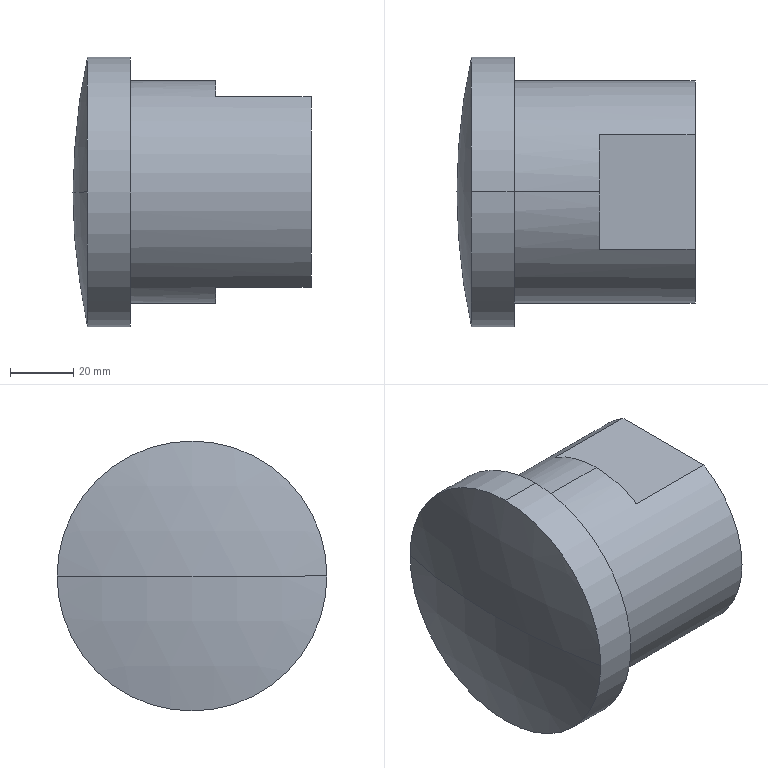Part | STEP file | OP10-028_cylinder connector (L) | 1 solid | 16 faces | box 75 x 85 x 85 mm | volume 251301 mm3 | cylinder 6 | plane 6 | cone 2 | sphere 2 | commonest cylinder face diameters 34.5 x2 70 x2 85 x2
STEP:
#1=CARTESIAN_POINT('',(0.,0.,0.));
#2=DIRECTION('',(0.,0.,1.));
#3=DIRECTION('',(1.,0.,0.));
#4=AXIS2_PLACEMENT_3D('',#1,#2,#3);
#5=CARTESIAN_POINT('',(-50.,0.,-17.25));
#6=VERTEX_POINT('',#5);
#7=CARTESIAN_POINT('',(0.,0.,-17.25));
#8=VERTEX_POINT('',#7);
#9=CARTESIAN_POINT('',(0.,0.,-17.25));
#10=DIRECTION('',(1.,0.,0.));
#11=VECTOR('',#10,1.);
#12=LINE('',#9,#11);
#13=CARTESIAN_POINT('',(0.,0.,0.));
#14=DIRECTION('',(1.,0.,0.));
#15=DIRECTION('',(0.,0.,-1.));
#16=AXIS2_PLACEMENT_3D('',#13,#14,#15);
#17=CYLINDRICAL_SURFACE('',#16,17.25);
#18=CARTESIAN_POINT('',(6.283,0.));
#19=DIRECTION('',(0.,1.));
#20=VECTOR('',#19,1.);
#21=LINE('',#18,#20);
#22=(GEOMETRIC_REPRESENTATION_CONTEXT(2)PARAMETRIC_REPRESENTATION_CONTEXT()REPRESENTATION_CONTEXT('',''));
#23=DEFINITIONAL_REPRESENTATION('',(#21),#22);
#24=PCURVE('',#17,#23);
#25=CARTESIAN_POINT('',(0.,0.,0.));
#26=DIRECTION('',(1.,0.,0.));
#27=DIRECTION('',(0.,0.,-1.));
#28=AXIS2_PLACEMENT_3D('',#25,#26,#27);
#29=CYLINDRICAL_SURFACE('',#28,17.25);
#30=CARTESIAN_POINT('',(0.,0.));
#31=DIRECTION('',(0.,1.));
#32=VECTOR('',#31,1.);
#33=LINE('',#30,#32);
#34=(GEOMETRIC_REPRESENTATION_CONTEXT(2)PARAMETRIC_REPRESENTATION_CONTEXT()REPRESENTATION_CONTEXT('',''));
#35=DEFINITIONAL_REPRESENTATION('',(#33),#34);
#36=PCURVE('',#29,#35);
#37=SURFACE_CURVE('',#12,(#24,#36),.PCURVE_S1.);
#38=EDGE_CURVE('',#6,#8,#37,.T.);
#39=ORIENTED_EDGE('',*,*,#38,.T.);
#40=CARTESIAN_POINT('',(0.,0.,17.25));
#41=VERTEX_POINT('',#40);
#42=CARTESIAN_POINT('',(0.,0.,0.));
#43=DIRECTION('',(1.,0.,0.));
#44=DIRECTION('',(0.,0.,-1.));
#45=AXIS2_PLACEMENT_3D('',#42,#43,#44);
#46=CIRCLE('',#45,17.25);
#47=CARTESIAN_POINT('',(0.,0.));
#48=DIRECTION('',(1.,0.));
#49=VECTOR('',#48,1.);
#50=LINE('',#47,#49);
#51=(GEOMETRIC_REPRESENTATION_CONTEXT(2)PARAMETRIC_REPRESENTATION_CONTEXT()REPRESENTATION_CONTEXT('',''));
#52=DEFINITIONAL_REPRESENTATION('',(#50),#51);
#53=PCURVE('',#17,#52);
#54=CARTESIAN_POINT('',(0.,0.,0.));
#55=DIRECTION('',(1.,0.,0.));
#56=DIRECTION('',(0.,0.,-1.));
#57=AXIS2_PLACEMENT_3D('',#54,#55,#56);
#58=PLANE('',#57);
#59=CARTESIAN_POINT('',(0.,0.));
#60=DIRECTION('',(1.,0.));
#61=AXIS2_PLACEMENT_2D('',#59,#60);
#62=CIRCLE('',#61,17.25);
#63=(GEOMETRIC_REPRESENTATION_CONTEXT(2)PARAMETRIC_REPRESENTATION_CONTEXT()REPRESENTATION_CONTEXT('',''));
#64=DEFINITIONAL_REPRESENTATION('',(#62),#63);
#65=PCURVE('',#58,#64);
#66=SURFACE_CURVE('',#46,(#53,#65),.PCURVE_S1.);
#67=EDGE_CURVE('',#41,#8,#66,.T.);
#68=ORIENTED_EDGE('',*,*,#67,.F.);
#69=CARTESIAN_POINT('',(-50.,0.,17.25));
#70=VERTEX_POINT('',#69);
#71=CARTESIAN_POINT('',(0.,0.,17.25));
#72=DIRECTION('',(1.,0.,0.));
#73=VECTOR('',#72,1.);
#74=LINE('',#71,#73);
#75=CARTESIAN_POINT('',(3.142,0.));
#76=DIRECTION('',(0.,1.));
#77=VECTOR('',#76,1.);
#78=LINE('',#75,#77);
#79=(GEOMETRIC_REPRESENTATION_CONTEXT(2)PARAMETRIC_REPRESENTATION_CONTEXT()REPRESENTATION_CONTEXT('',''));
#80=DEFINITIONAL_REPRESENTATION('',(#78),#79);
#81=PCURVE('',#17,#80);
#82=CARTESIAN_POINT('',(3.142,0.));
#83=DIRECTION('',(0.,1.));
#84=VECTOR('',#83,1.);
#85=LINE('',#82,#84);
#86=(GEOMETRIC_REPRESENTATION_CONTEXT(2)PARAMETRIC_REPRESENTATION_CONTEXT()REPRESENTATION_CONTEXT('',''));
#87=DEFINITIONAL_REPRESENTATION('',(#85),#86);
#88=PCURVE('',#29,#87);
#89=SURFACE_CURVE('',#74,(#81,#88),.PCURVE_S1.);
#90=EDGE_CURVE('',#70,#41,#89,.T.);
#91=ORIENTED_EDGE('',*,*,#90,.F.);
#92=CARTESIAN_POINT('',(-50.,0.,0.));
#93=DIRECTION('',(1.,0.,0.));
#94=DIRECTION('',(0.,0.,-1.));
#95=AXIS2_PLACEMENT_3D('',#92,#93,#94);
#96=CIRCLE('',#95,17.25);
#97=CARTESIAN_POINT('',(0.,-50.));
#98=DIRECTION('',(1.,0.));
#99=VECTOR('',#98,1.);
#100=LINE('',#97,#99);
#101=(GEOMETRIC_REPRESENTATION_CONTEXT(2)PARAMETRIC_REPRESENTATION_CONTEXT()REPRESENTATION_CONTEXT('',''));
#102=DEFINITIONAL_REPRESENTATION('',(#100),#101);
#103=PCURVE('',#17,#102);
#104=CARTESIAN_POINT('',(-50.,0.,0.));
#105=DIRECTION('',(1.,0.,0.));
#106=DIRECTION('',(0.,0.,-1.));
#107=AXIS2_PLACEMENT_3D('',#104,#105,#106);
#108=CONICAL_SURFACE('',#107,17.25,1.03);
#109=CARTESIAN_POINT('',(0.,0.));
#110=DIRECTION('',(1.,0.));
#111=VECTOR('',#110,1.);
#112=LINE('',#109,#111);
#113=(GEOMETRIC_REPRESENTATION_CONTEXT(2)PARAMETRIC_REPRESENTATION_CONTEXT()REPRESENTATION_CONTEXT('',''));
#114=DEFINITIONAL_REPRESENTATION('',(#112),#113);
#115=PCURVE('',#108,#114);
#116=SURFACE_CURVE('',#96,(#103,#115),.PCURVE_S1.);
#117=EDGE_CURVE('',#70,#6,#116,.T.);
#118=ORIENTED_EDGE('',*,*,#117,.T.);
#119=EDGE_LOOP('',(#39,#68,#91,#118));
#120=FACE_BOUND('',#119,.F.);
#121=ADVANCED_FACE('',(#120),#17,.F.);
#122=ORIENTED_EDGE('',*,*,#117,.F.);
#123=CARTESIAN_POINT('',(-60.365,0.,0.));
#124=VERTEX_POINT('',#123);
#125=CARTESIAN_POINT('',(-50.,0.,17.25));
#126=DIRECTION('',(0.515,0.,0.8572));
#127=VECTOR('',#126,1.);
#128=LINE('',#125,#127);
#129=CARTESIAN_POINT('',(3.142,0.));
#130=DIRECTION('',(0.,1.));
#131=VECTOR('',#130,1.);
#132=LINE('',#129,#131);
#133=(GEOMETRIC_REPRESENTATION_CONTEXT(2)PARAMETRIC_REPRESENTATION_CONTEXT()REPRESENTATION_CONTEXT('',''));
#134=DEFINITIONAL_REPRESENTATION('',(#132),#133);
#135=PCURVE('',#108,#134);
#136=CARTESIAN_POINT('',(-50.,0.,0.));
#137=DIRECTION('',(1.,0.,0.));
#138=DIRECTION('',(0.,0.,-1.));
#139=AXIS2_PLACEMENT_3D('',#136,#137,#138);
#140=CONICAL_SURFACE('',#139,17.25,1.03);
#141=CARTESIAN_POINT('',(3.142,0.));
#142=DIRECTION('',(0.,1.));
#143=VECTOR('',#142,1.);
#144=LINE('',#141,#143);
#145=(GEOMETRIC_REPRESENTATION_CONTEXT(2)PARAMETRIC_REPRESENTATION_CONTEXT()REPRESENTATION_CONTEXT('',''));
#146=DEFINITIONAL_REPRESENTATION('',(#144),#145);
#147=PCURVE('',#140,#146);
#148=SURFACE_CURVE('',#128,(#135,#147),.PCURVE_S1.);
#149=EDGE_CURVE('',#124,#70,#148,.T.);
#150=ORIENTED_EDGE('',*,*,#149,.F.);
#151=CARTESIAN_POINT('',(-50.,0.,-17.25));
#152=DIRECTION('',(0.515,0.,-0.8572));
#153=VECTOR('',#152,1.);
#154=LINE('',#151,#153);
#155=CARTESIAN_POINT('',(6.283,0.));
#156=DIRECTION('',(0.,1.));
#157=VECTOR('',#156,1.);
#158=LINE('',#155,#157);
#159=(GEOMETRIC_REPRESENTATION_CONTEXT(2)PARAMETRIC_REPRESENTATION_CONTEXT()REPRESENTATION_CONTEXT('',''));
#160=DEFINITIONAL_REPRESENTATION('',(#158),#159);
#161=PCURVE('',#108,#160);
#162=CARTESIAN_POINT('',(0.,0.));
#163=DIRECTION('',(0.,1.));
#164=VECTOR('',#163,1.);
#165=LINE('',#162,#164);
#166=(GEOMETRIC_REPRESENTATION_CONTEXT(2)PARAMETRIC_REPRESENTATION_CONTEXT()REPRESENTATION_CONTEXT('',''));
#167=DEFINITIONAL_REPRESENTATION('',(#165),#166);
#168=PCURVE('',#140,#167);
#169=SURFACE_CURVE('',#154,(#161,#168),.PCURVE_S1.);
#170=EDGE_CURVE('',#124,#6,#169,.T.);
#171=ORIENTED_EDGE('',*,*,#170,.T.);
#172=EDGE_LOOP('',(#122,#150,#171));
#173=FACE_BOUND('',#172,.F.);
#174=ADVANCED_FACE('',(#173),#108,.F.);
#175=CARTESIAN_POINT('',(-75.,0.,0.));
#176=VERTEX_POINT('',#175);
#177=CARTESIAN_POINT('',(-70.432,42.5,0.));
#178=VERTEX_POINT('',#177);
#179=CARTESIAN_POINT('',(125.,0.,0.));
#180=DIRECTION('',(0.,0.,-1.));
#181=DIRECTION('',(-1.,0.,0.));
#182=AXIS2_PLACEMENT_3D('',#179,#180,#181);
#183=CIRCLE('',#182,200.);
#184=CARTESIAN_POINT('',(125.,0.,0.));
#185=DIRECTION('',(0.,0.,1.));
#186=DIRECTION('',(0.,1.,0.));
#187=AXIS2_PLACEMENT_3D('',#184,#185,#186);
#188=SPHERICAL_SURFACE('',#187,200.);
#189=CARTESIAN_POINT('',(1.571,0.));
#190=DIRECTION('',(-1.,0.));
#191=VECTOR('',#190,1.);
#192=LINE('',#189,#191);
#193=(GEOMETRIC_REPRESENTATION_CONTEXT(2)PARAMETRIC_REPRESENTATION_CONTEXT()REPRESENTATION_CONTEXT('',''));
#194=DEFINITIONAL_REPRESENTATION('',(#192),#193);
#195=PCURVE('',#188,#194);
#196=CARTESIAN_POINT('',(125.,0.,0.));
#197=DIRECTION('',(0.,0.,1.));
#198=DIRECTION('',(0.,1.,0.));
#199=AXIS2_PLACEMENT_3D('',#196,#197,#198);
#200=SPHERICAL_SURFACE('',#199,200.);
#201=CARTESIAN_POINT('',(1.571,0.));
#202=DIRECTION('',(-1.,0.));
#203=VECTOR('',#202,1.);
#204=LINE('',#201,#203);
#205=(GEOMETRIC_REPRESENTATION_CONTEXT(2)PARAMETRIC_REPRESENTATION_CONTEXT()REPRESENTATION_CONTEXT('',''));
#206=DEFINITIONAL_REPRESENTATION('',(#204),#205);
#207=PCURVE('',#200,#206);
#208=SURFACE_CURVE('',#183,(#195,#207),.PCURVE_S1.);
#209=EDGE_CURVE('',#176,#178,#208,.T.);
#210=ORIENTED_EDGE('',*,*,#209,.F.);
#211=CARTESIAN_POINT('',(-70.432,-42.5,0.));
#212=VERTEX_POINT('',#211);
#213=CARTESIAN_POINT('',(125.,0.,0.));
#214=DIRECTION('',(0.,0.,1.));
#215=DIRECTION('',(0.,-1.,0.));
#216=AXIS2_PLACEMENT_3D('',#213,#214,#215);
#217=CIRCLE('',#216,200.);
#218=CARTESIAN_POINT('',(-3.142,0.));
#219=DIRECTION('',(1.,0.));
#220=VECTOR('',#219,1.);
#221=LINE('',#218,#220);
#222=(GEOMETRIC_REPRESENTATION_CONTEXT(2)PARAMETRIC_REPRESENTATION_CONTEXT()REPRESENTATION_CONTEXT('',''));
#223=DEFINITIONAL_REPRESENTATION('',(#221),#222);
#224=PCURVE('',#188,#223);
#225=CARTESIAN_POINT('',(-3.142,0.));
#226=DIRECTION('',(1.,0.));
#227=VECTOR('',#226,1.);
#228=LINE('',#225,#227);
#229=(GEOMETRIC_REPRESENTATION_CONTEXT(2)PARAMETRIC_REPRESENTATION_CONTEXT()REPRESENTATION_CONTEXT('',''));
#230=DEFINITIONAL_REPRESENTATION('',(#228),#229);
#231=PCURVE('',#200,#230);
#232=SURFACE_CURVE('',#217,(#224,#231),.PCURVE_S1.);
#233=EDGE_CURVE('',#176,#212,#232,.T.);
#234=ORIENTED_EDGE('',*,*,#233,.T.);
#235=CARTESIAN_POINT('',(-70.432,0.,42.5));
#236=VERTEX_POINT('',#235);
#237=CARTESIAN_POINT('',(-70.432,0.,0.));
#238=DIRECTION('',(1.,0.,0.));
#239=DIRECTION('',(0.,0.,-1.));
#240=AXIS2_PLACEMENT_3D('',#237,#238,#239);
#241=CIRCLE('',#240,42.5);
#242=CARTESIAN_POINT('',(1.571,0.2141));
#243=CARTESIAN_POINT('',(1.576,0.2141));
#244=CARTESIAN_POINT('',(1.586,0.2138));
#245=CARTESIAN_POINT('',(1.602,0.2121));
#246=CARTESIAN_POINT('',(1.617,0.2093));
#247=CARTESIAN_POINT('',(1.632,0.2055));
#248=CARTESIAN_POINT('',(1.647,0.2006));
#249=CARTESIAN_POINT('',(1.661,0.1947));
#250=CARTESIAN_POINT('',(1.675,0.1878));
#251=CARTESIAN_POINT('',(1.688,0.1799));
#252=CARTESIAN_POINT('',(1.701,0.1711));
#253=CARTESIAN_POINT('',(1.712,0.1614));
#254=CARTESIAN_POINT('',(1.724,0.151));
#255=CARTESIAN_POINT('',(1.734,0.1397));
#256=CARTESIAN_POINT('',(1.743,0.1278));
#257=CARTESIAN_POINT('',(1.752,0.1152));
#258=CARTESIAN_POINT('',(1.76,0.1021));
#259=CARTESIAN_POINT('',(1.766,0.08846));
#260=CARTESIAN_POINT('',(1.772,0.07439));
#261=CARTESIAN_POINT('',(1.777,0.05995));
#262=CARTESIAN_POINT('',(1.78,0.04522));
#263=CARTESIAN_POINT('',(1.783,0.03027));
#264=CARTESIAN_POINT('',(1.785,0.01517));
#265=CARTESIAN_POINT('',(1.785,0.005058));
#266=CARTESIAN_POINT('',(1.785,0.));
#267=B_SPLINE_CURVE_WITH_KNOTS('',3,(#242,#243,#244,#245,#246,#247,#248,#249,#250,#251,#252,#253,#254,#255,#256,#257,#258,#259,#260,#261,#262,#263,#264,#265,#266),.UNSPECIFIED.,.F.,.F.,(4,1,1,1,1,1,1,1,1,1,1,1,1,1,1,1,1,1,1,1,1,1,4),(3.142,3.213,3.284,3.356,3.427,3.499,3.57,3.641,3.713,3.784,3.856,3.927,3.998,4.07,4.141,4.213,4.284,4.355,4.427,4.498,4.57,4.641,4.712),.QUASI_UNIFORM_KNOTS.);
#268=(GEOMETRIC_REPRESENTATION_CONTEXT(2)PARAMETRIC_REPRESENTATION_CONTEXT()REPRESENTATION_CONTEXT('',''));
#269=DEFINITIONAL_REPRESENTATION('',(#267),#268);
#270=PCURVE('',#188,#269);
#271=CARTESIAN_POINT('',(0.,0.,0.));
#272=DIRECTION('',(1.,0.,0.));
#273=DIRECTION('',(0.,0.,-1.));
#274=AXIS2_PLACEMENT_3D('',#271,#272,#273);
#275=CYLINDRICAL_SURFACE('',#274,42.5);
#276=CARTESIAN_POINT('',(0.,-70.432));
#277=DIRECTION('',(1.,0.));
#278=VECTOR('',#277,1.);
#279=LINE('',#276,#278);
#280=(GEOMETRIC_REPRESENTATION_CONTEXT(2)PARAMETRIC_REPRESENTATION_CONTEXT()REPRESENTATION_CONTEXT('',''));
#281=DEFINITIONAL_REPRESENTATION('',(#279),#280);
#282=PCURVE('',#275,#281);
#283=SURFACE_CURVE('',#241,(#270,#282),.PCURVE_S1.);
#284=EDGE_CURVE('',#236,#212,#283,.T.);
#285=ORIENTED_EDGE('',*,*,#284,.F.);
#286=CARTESIAN_POINT('',(-70.432,0.,0.));
#287=DIRECTION('',(1.,0.,0.));
#288=DIRECTION('',(0.,0.,-1.));
#289=AXIS2_PLACEMENT_3D('',#286,#287,#288);
#290=CIRCLE('',#289,42.5);
#291=CARTESIAN_POINT('',(1.357,0.));
#292=CARTESIAN_POINT('',(1.357,0.005058));
#293=CARTESIAN_POINT('',(1.357,0.01517));
#294=CARTESIAN_POINT('',(1.359,0.03027));
#295=CARTESIAN_POINT('',(1.361,0.04522));
#296=CARTESIAN_POINT('',(1.365,0.05995));
#297=CARTESIAN_POINT('',(1.37,0.07439));
#298=CARTESIAN_POINT('',(1.375,0.08846));
#299=CARTESIAN_POINT('',(1.382,0.1021));
#300=CARTESIAN_POINT('',(1.39,0.1152));
#301=CARTESIAN_POINT('',(1.398,0.1278));
#302=CARTESIAN_POINT('',(1.408,0.1397));
#303=CARTESIAN_POINT('',(1.418,0.151));
#304=CARTESIAN_POINT('',(1.429,0.1614));
#305=CARTESIAN_POINT('',(1.441,0.1711));
#306=CARTESIAN_POINT('',(1.454,0.1799));
#307=CARTESIAN_POINT('',(1.467,0.1878));
#308=CARTESIAN_POINT('',(1.481,0.1947));
#309=CARTESIAN_POINT('',(1.495,0.2006));
#310=CARTESIAN_POINT('',(1.51,0.2055));
#311=CARTESIAN_POINT('',(1.525,0.2093));
#312=CARTESIAN_POINT('',(1.54,0.2121));
#313=CARTESIAN_POINT('',(1.555,0.2138));
#314=CARTESIAN_POINT('',(1.566,0.2141));
#315=CARTESIAN_POINT('',(1.571,0.2141));
#316=B_SPLINE_CURVE_WITH_KNOTS('',3,(#291,#292,#293,#294,#295,#296,#297,#298,#299,#300,#301,#302,#303,#304,#305,#306,#307,#308,#309,#310,#311,#312,#313,#314,#315),.UNSPECIFIED.,.F.,.F.,(4,1,1,1,1,1,1,1,1,1,1,1,1,1,1,1,1,1,1,1,1,1,4),(1.571,1.642,1.714,1.785,1.856,1.928,1.999,2.071,2.142,2.213,2.285,2.356,2.428,2.499,2.57,2.642,2.713,2.785,2.856,2.927,2.999,3.07,3.142),.QUASI_UNIFORM_KNOTS.);
#317=(GEOMETRIC_REPRESENTATION_CONTEXT(2)PARAMETRIC_REPRESENTATION_CONTEXT()REPRESENTATION_CONTEXT('',''));
#318=DEFINITIONAL_REPRESENTATION('',(#316),#317);
#319=PCURVE('',#188,#318);
#320=CARTESIAN_POINT('',(0.,0.,0.));
#321=DIRECTION('',(1.,0.,0.));
#322=DIRECTION('',(0.,0.,-1.));
#323=AXIS2_PLACEMENT_3D('',#320,#321,#322);
#324=CYLINDRICAL_SURFACE('',#323,42.5);
#325=CARTESIAN_POINT('',(0.,-70.432));
#326=DIRECTION('',(1.,0.));
#327=VECTOR('',#326,1.);
#328=LINE('',#325,#327);
#329=(GEOMETRIC_REPRESENTATION_CONTEXT(2)PARAMETRIC_REPRESENTATION_CONTEXT()REPRESENTATION_CONTEXT('',''));
#330=DEFINITIONAL_REPRESENTATION('',(#328),#329);
#331=PCURVE('',#324,#330);
#332=SURFACE_CURVE('',#290,(#319,#331),.PCURVE_S1.);
#333=EDGE_CURVE('',#178,#236,#332,.T.);
#334=ORIENTED_EDGE('',*,*,#333,.F.);
#335=EDGE_LOOP('',(#210,#234,#285,#334));
#336=FACE_BOUND('',#335,.T.);
#337=ADVANCED_FACE('',(#336),#188,.T.);
#338=CARTESIAN_POINT('',(-70.432,0.,-42.5));
#339=VERTEX_POINT('',#338);
#340=CARTESIAN_POINT('',(-70.432,0.,0.));
#341=DIRECTION('',(1.,0.,0.));
#342=DIRECTION('',(0.,0.,-1.));
#343=AXIS2_PLACEMENT_3D('',#340,#341,#342);
#344=CIRCLE('',#343,42.5);
#345=CARTESIAN_POINT('',(0.,-70.432));
#346=DIRECTION('',(1.,0.));
#347=VECTOR('',#346,1.);
#348=LINE('',#345,#347);
#349=(GEOMETRIC_REPRESENTATION_CONTEXT(2)PARAMETRIC_REPRESENTATION_CONTEXT()REPRESENTATION_CONTEXT('',''));
#350=DEFINITIONAL_REPRESENTATION('',(#348),#349);
#351=PCURVE('',#324,#350);
#352=CARTESIAN_POINT('',(1.571,-0.2141));
#353=CARTESIAN_POINT('',(1.566,-0.2141));
#354=CARTESIAN_POINT('',(1.555,-0.2138));
#355=CARTESIAN_POINT('',(1.54,-0.2121));
#356=CARTESIAN_POINT('',(1.525,-0.2093));
#357=CARTESIAN_POINT('',(1.51,-0.2055));
#358=CARTESIAN_POINT('',(1.495,-0.2006));
#359=CARTESIAN_POINT('',(1.481,-0.1947));
#360=CARTESIAN_POINT('',(1.467,-0.1878));
#361=CARTESIAN_POINT('',(1.454,-0.1799));
#362=CARTESIAN_POINT('',(1.441,-0.1711));
#363=CARTESIAN_POINT('',(1.429,-0.1614));
#364=CARTESIAN_POINT('',(1.418,-0.151));
#365=CARTESIAN_POINT('',(1.408,-0.1397));
#366=CARTESIAN_POINT('',(1.398,-0.1278));
#367=CARTESIAN_POINT('',(1.39,-0.1152));
#368=CARTESIAN_POINT('',(1.382,-0.1021));
#369=CARTESIAN_POINT('',(1.375,-0.08846));
#370=CARTESIAN_POINT('',(1.37,-0.07439));
#371=CARTESIAN_POINT('',(1.365,-0.05995));
#372=CARTESIAN_POINT('',(1.361,-0.04522));
#373=CARTESIAN_POINT('',(1.359,-0.03027));
#374=CARTESIAN_POINT('',(1.357,-0.01517));
#375=CARTESIAN_POINT('',(1.357,-0.005058));
#376=CARTESIAN_POINT('',(1.357,0.));
#377=B_SPLINE_CURVE_WITH_KNOTS('',3,(#352,#353,#354,#355,#356,#357,#358,#359,#360,#361,#362,#363,#364,#365,#366,#367,#368,#369,#370,#371,#372,#373,#374,#375,#376),.UNSPECIFIED.,.F.,.F.,(4,1,1,1,1,1,1,1,1,1,1,1,1,1,1,1,1,1,1,1,1,1,4),(0.,0.0714,0.1428,0.2142,0.2856,0.357,0.4284,0.4998,0.5712,0.6426,0.714,0.7854,0.8568,0.9282,0.9996,1.071,1.142,1.214,1.285,1.357,1.428,1.499,1.571),.QUASI_UNIFORM_KNOTS.);
#378=(GEOMETRIC_REPRESENTATION_CONTEXT(2)PARAMETRIC_REPRESENTATION_CONTEXT()REPRESENTATION_CONTEXT('',''));
#379=DEFINITIONAL_REPRESENTATION('',(#377),#378);
#380=PCURVE('',#200,#379);
#381=SURFACE_CURVE('',#344,(#351,#380),.PCURVE_S1.);
#382=EDGE_CURVE('',#339,#178,#381,.T.);
#383=ORIENTED_EDGE('',*,*,#382,.T.);
#384=ORIENTED_EDGE('',*,*,#333,.T.);
#385=CARTESIAN_POINT('',(-57.,0.,42.5));
#386=VERTEX_POINT('',#385);
#387=CARTESIAN_POINT('',(0.,0.,42.5));
#388=DIRECTION('',(1.,0.,0.));
#389=VECTOR('',#388,1.);
#390=LINE('',#387,#389);
#391=CARTESIAN_POINT('',(3.142,0.));
#392=DIRECTION('',(0.,1.));
#393=VECTOR('',#392,1.);
#394=LINE('',#391,#393);
#395=(GEOMETRIC_REPRESENTATION_CONTEXT(2)PARAMETRIC_REPRESENTATION_CONTEXT()REPRESENTATION_CONTEXT('',''));
#396=DEFINITIONAL_REPRESENTATION('',(#394),#395);
#397=PCURVE('',#324,#396);
#398=CARTESIAN_POINT('',(3.142,0.));
#399=DIRECTION('',(0.,1.));
#400=VECTOR('',#399,1.);
#401=LINE('',#398,#400);
#402=(GEOMETRIC_REPRESENTATION_CONTEXT(2)PARAMETRIC_REPRESENTATION_CONTEXT()REPRESENTATION_CONTEXT('',''));
#403=DEFINITIONAL_REPRESENTATION('',(#401),#402);
#404=PCURVE('',#275,#403);
#405=SURFACE_CURVE('',#390,(#397,#404),.PCURVE_S1.);
#406=EDGE_CURVE('',#236,#386,#405,.T.);
#407=ORIENTED_EDGE('',*,*,#406,.T.);
#408=CARTESIAN_POINT('',(-57.,0.,-42.5));
#409=VERTEX_POINT('',#408);
#410=CARTESIAN_POINT('',(-57.,0.,0.));
#411=DIRECTION('',(1.,0.,0.));
#412=DIRECTION('',(0.,0.,-1.));
#413=AXIS2_PLACEMENT_3D('',#410,#411,#412);
#414=CIRCLE('',#413,42.5);
#415=CARTESIAN_POINT('',(0.,-57.));
#416=DIRECTION('',(1.,0.));
#417=VECTOR('',#416,1.);
#418=LINE('',#415,#417);
#419=(GEOMETRIC_REPRESENTATION_CONTEXT(2)PARAMETRIC_REPRESENTATION_CONTEXT()REPRESENTATION_CONTEXT('',''));
#420=DEFINITIONAL_REPRESENTATION('',(#418),#419);
#421=PCURVE('',#324,#420);
#422=CARTESIAN_POINT('',(-57.,35.,0.));
#423=DIRECTION('',(1.,0.,0.));
#424=DIRECTION('',(0.,0.,-1.));
#425=AXIS2_PLACEMENT_3D('',#422,#423,#424);
#426=PLANE('',#425);
#427=CARTESIAN_POINT('',(0.,-35.));
#428=DIRECTION('',(1.,0.));
#429=AXIS2_PLACEMENT_2D('',#427,#428);
#430=CIRCLE('',#429,42.5);
#431=(GEOMETRIC_REPRESENTATION_CONTEXT(2)PARAMETRIC_REPRESENTATION_CONTEXT()REPRESENTATION_CONTEXT('',''));
#432=DEFINITIONAL_REPRESENTATION('',(#430),#431);
#433=PCURVE('',#426,#432);
#434=SURFACE_CURVE('',#414,(#421,#433),.PCURVE_S1.);
#435=EDGE_CURVE('',#409,#386,#434,.T.);
#436=ORIENTED_EDGE('',*,*,#435,.F.);
#437=CARTESIAN_POINT('',(0.,0.,-42.5));
#438=DIRECTION('',(1.,0.,0.));
#439=VECTOR('',#438,1.);
#440=LINE('',#437,#439);
#441=CARTESIAN_POINT('',(0.,0.));
#442=DIRECTION('',(0.,1.));
#443=VECTOR('',#442,1.);
#444=LINE('',#441,#443);
#445=(GEOMETRIC_REPRESENTATION_CONTEXT(2)PARAMETRIC_REPRESENTATION_CONTEXT()REPRESENTATION_CONTEXT('',''));
#446=DEFINITIONAL_REPRESENTATION('',(#444),#445);
#447=PCURVE('',#324,#446);
#448=CARTESIAN_POINT('',(6.283,0.));
#449=DIRECTION('',(0.,1.));
#450=VECTOR('',#449,1.);
#451=LINE('',#448,#450);
#452=(GEOMETRIC_REPRESENTATION_CONTEXT(2)PARAMETRIC_REPRESENTATION_CONTEXT()REPRESENTATION_CONTEXT('',''));
#453=DEFINITIONAL_REPRESENTATION('',(#451),#452);
#454=PCURVE('',#275,#453);
#455=SURFACE_CURVE('',#440,(#447,#454),.PCURVE_S1.);
#456=EDGE_CURVE('',#339,#409,#455,.T.);
#457=ORIENTED_EDGE('',*,*,#456,.F.);
#458=EDGE_LOOP('',(#383,#384,#407,#436,#457));
#459=FACE_BOUND('',#458,.T.);
#460=ADVANCED_FACE('',(#459),#324,.T.);
#461=CARTESIAN_POINT('',(-57.,0.,-35.));
#462=VERTEX_POINT('',#461);
#463=CARTESIAN_POINT('',(-57.,0.,35.));
#464=VERTEX_POINT('',#463);
#465=CARTESIAN_POINT('',(-57.,0.,0.));
#466=DIRECTION('',(1.,0.,0.));
#467=DIRECTION('',(0.,0.,-1.));
#468=AXIS2_PLACEMENT_3D('',#465,#466,#467);
#469=CIRCLE('',#468,35.);
#470=CARTESIAN_POINT('',(0.,0.,0.));
#471=DIRECTION('',(1.,0.,0.));
#472=DIRECTION('',(0.,0.,-1.));
#473=AXIS2_PLACEMENT_3D('',#470,#471,#472);
#474=CYLINDRICAL_SURFACE('',#473,35.);
#475=CARTESIAN_POINT('',(0.,-57.));
#476=DIRECTION('',(1.,0.));
#477=VECTOR('',#476,1.);
#478=LINE('',#475,#477);
#479=(GEOMETRIC_REPRESENTATION_CONTEXT(2)PARAMETRIC_REPRESENTATION_CONTEXT()REPRESENTATION_CONTEXT('',''));
#480=DEFINITIONAL_REPRESENTATION('',(#478),#479);
#481=PCURVE('',#474,#480);
#482=CARTESIAN_POINT('',(0.,-35.));
#483=DIRECTION('',(1.,0.));
#484=AXIS2_PLACEMENT_2D('',#482,#483);
#485=CIRCLE('',#484,35.);
#486=(GEOMETRIC_REPRESENTATION_CONTEXT(2)PARAMETRIC_REPRESENTATION_CONTEXT()REPRESENTATION_CONTEXT('',''));
#487=DEFINITIONAL_REPRESENTATION('',(#485),#486);
#488=PCURVE('',#426,#487);
#489=SURFACE_CURVE('',#469,(#481,#488),.PCURVE_S1.);
#490=EDGE_CURVE('',#462,#464,#489,.T.);
#491=ORIENTED_EDGE('',*,*,#490,.T.);
#492=CARTESIAN_POINT('',(-30.,0.,35.));
#493=VERTEX_POINT('',#492);
#494=CARTESIAN_POINT('',(0.,0.,35.));
#495=DIRECTION('',(1.,0.,0.));
#496=VECTOR('',#495,1.);
#497=LINE('',#494,#496);
#498=CARTESIAN_POINT('',(3.142,0.));
#499=DIRECTION('',(0.,1.));
#500=VECTOR('',#499,1.);
#501=LINE('',#498,#500);
#502=(GEOMETRIC_REPRESENTATION_CONTEXT(2)PARAMETRIC_REPRESENTATION_CONTEXT()REPRESENTATION_CONTEXT('',''));
#503=DEFINITIONAL_REPRESENTATION('',(#501),#502);
#504=PCURVE('',#474,#503);
#505=CARTESIAN_POINT('',(0.,0.,0.));
#506=DIRECTION('',(1.,0.,0.));
#507=DIRECTION('',(0.,0.,-1.));
#508=AXIS2_PLACEMENT_3D('',#505,#506,#507);
#509=CYLINDRICAL_SURFACE('',#508,35.);
#510=CARTESIAN_POINT('',(3.142,0.));
#511=DIRECTION('',(0.,1.));
#512=VECTOR('',#511,1.);
#513=LINE('',#510,#512);
#514=(GEOMETRIC_REPRESENTATION_CONTEXT(2)PARAMETRIC_REPRESENTATION_CONTEXT()REPRESENTATION_CONTEXT('',''));
#515=DEFINITIONAL_REPRESENTATION('',(#513),#514);
#516=PCURVE('',#509,#515);
#517=SURFACE_CURVE('',#497,(#504,#516),.PCURVE_S1.);
#518=EDGE_CURVE('',#464,#493,#517,.T.);
#519=ORIENTED_EDGE('',*,*,#518,.T.);
#520=CARTESIAN_POINT('',(-30.,18.028,30.));
#521=VERTEX_POINT('',#520);
#522=CARTESIAN_POINT('',(-30.,0.,0.));
#523=DIRECTION('',(-1.,0.,0.));
#524=DIRECTION('',(0.,0.,-1.));
#525=AXIS2_PLACEMENT_3D('',#522,#523,#524);
#526=CIRCLE('',#525,35.);
#527=CARTESIAN_POINT('',(6.283,-30.));
#528=DIRECTION('',(-1.,0.));
#529=VECTOR('',#528,1.);
#530=LINE('',#527,#529);
#531=(GEOMETRIC_REPRESENTATION_CONTEXT(2)PARAMETRIC_REPRESENTATION_CONTEXT()REPRESENTATION_CONTEXT('',''));
#532=DEFINITIONAL_REPRESENTATION('',(#530),#531);
#533=PCURVE('',#474,#532);
#534=CARTESIAN_POINT('',(-30.,-35.,40.));
#535=DIRECTION('',(1.,0.,0.));
#536=DIRECTION('',(0.,0.,-1.));
#537=AXIS2_PLACEMENT_3D('',#534,#535,#536);
#538=PLANE('',#537);
#539=CARTESIAN_POINT('',(75.,35.));
#540=CARTESIAN_POINT('',(75.,-25.622));
#541=CARTESIAN_POINT('',(22.5,4.689));
#542=CARTESIAN_POINT('',(-30.,35.));
#543=CARTESIAN_POINT('',(22.5,65.311));
#544=CARTESIAN_POINT('',(75.,95.622));
#545=CARTESIAN_POINT('',(75.,35.));
#546=(BOUNDED_CURVE()B_SPLINE_CURVE(2,(#539,#540,#541,#542,#543,#544,#545),.UNSPECIFIED.,.T.,.F.)B_SPLINE_CURVE_WITH_KNOTS((1,2,2,2,2,1),(-2.094,0.,2.094,4.189,6.283,8.378),.UNSPECIFIED.)CURVE()GEOMETRIC_REPRESENTATION_ITEM()RATIONAL_B_SPLINE_CURVE((1.,0.5,1.,0.5,1.,0.5,1.))REPRESENTATION_ITEM(''));
#547=(GEOMETRIC_REPRESENTATION_CONTEXT(2)PARAMETRIC_REPRESENTATION_CONTEXT()REPRESENTATION_CONTEXT('',''));
#548=DEFINITIONAL_REPRESENTATION('',(#546),#547);
#549=PCURVE('',#538,#548);
#550=SURFACE_CURVE('',#526,(#533,#549),.PCURVE_S1.);
#551=EDGE_CURVE('',#493,#521,#550,.T.);
#552=ORIENTED_EDGE('',*,*,#551,.T.);
#553=CARTESIAN_POINT('',(0.,18.028,30.));
#554=VERTEX_POINT('',#553);
#555=CARTESIAN_POINT('',(0.,18.028,30.));
#556=DIRECTION('',(-1.,0.,0.));
#557=VECTOR('',#556,1.);
#558=LINE('',#555,#557);
#559=CARTESIAN_POINT('',(2.6,0.));
#560=DIRECTION('',(0.,-1.));
#561=VECTOR('',#560,1.);
#562=LINE('',#559,#561);
#563=(GEOMETRIC_REPRESENTATION_CONTEXT(2)PARAMETRIC_REPRESENTATION_CONTEXT()REPRESENTATION_CONTEXT('',''));
#564=DEFINITIONAL_REPRESENTATION('',(#562),#563);
#565=PCURVE('',#474,#564);
#566=CARTESIAN_POINT('',(0.,0.,30.));
#567=DIRECTION('',(0.,0.,-1.));
#568=DIRECTION('',(-1.,0.,0.));
#569=AXIS2_PLACEMENT_3D('',#566,#567,#568);
#570=PLANE('',#569);
#571=CARTESIAN_POINT('',(0.,18.028));
#572=DIRECTION('',(1.,0.));
#573=VECTOR('',#572,1.);
#574=LINE('',#571,#573);
#575=(GEOMETRIC_REPRESENTATION_CONTEXT(2)PARAMETRIC_REPRESENTATION_CONTEXT()REPRESENTATION_CONTEXT('',''));
#576=DEFINITIONAL_REPRESENTATION('',(#574),#575);
#577=PCURVE('',#570,#576);
#578=SURFACE_CURVE('',#558,(#565,#577),.PCURVE_S1.);
#579=EDGE_CURVE('',#554,#521,#578,.T.);
#580=ORIENTED_EDGE('',*,*,#579,.F.);
#581=CARTESIAN_POINT('',(0.,18.028,-30.));
#582=VERTEX_POINT('',#581);
#583=CARTESIAN_POINT('',(0.,0.,0.));
#584=DIRECTION('',(1.,0.,0.));
#585=DIRECTION('',(0.,0.,-1.));
#586=AXIS2_PLACEMENT_3D('',#583,#584,#585);
#587=CIRCLE('',#586,35.);
#588=CARTESIAN_POINT('',(0.,0.));
#589=DIRECTION('',(1.,0.));
#590=VECTOR('',#589,1.);
#591=LINE('',#588,#590);
#592=(GEOMETRIC_REPRESENTATION_CONTEXT(2)PARAMETRIC_REPRESENTATION_CONTEXT()REPRESENTATION_CONTEXT('',''));
#593=DEFINITIONAL_REPRESENTATION('',(#591),#592);
#594=PCURVE('',#474,#593);
#595=CARTESIAN_POINT('',(0.,0.));
#596=DIRECTION('',(1.,0.));
#597=AXIS2_PLACEMENT_2D('',#595,#596);
#598=CIRCLE('',#597,35.);
#599=(GEOMETRIC_REPRESENTATION_CONTEXT(2)PARAMETRIC_REPRESENTATION_CONTEXT()REPRESENTATION_CONTEXT('',''));
#600=DEFINITIONAL_REPRESENTATION('',(#598),#599);
#601=PCURVE('',#58,#600);
#602=SURFACE_CURVE('',#587,(#594,#601),.PCURVE_S1.);
#603=EDGE_CURVE('',#582,#554,#602,.T.);
#604=ORIENTED_EDGE('',*,*,#603,.F.);
#605=CARTESIAN_POINT('',(-30.,18.028,-30.));
#606=VERTEX_POINT('',#605);
#607=CARTESIAN_POINT('',(0.,18.028,-30.));
#608=DIRECTION('',(1.,0.,0.));
#609=VECTOR('',#608,1.);
#610=LINE('',#607,#609);
#611=CARTESIAN_POINT('',(0.5411,0.));
#612=DIRECTION('',(0.,1.));
#613=VECTOR('',#612,1.);
#614=LINE('',#611,#613);
#615=(GEOMETRIC_REPRESENTATION_CONTEXT(2)PARAMETRIC_REPRESENTATION_CONTEXT()REPRESENTATION_CONTEXT('',''));
#616=DEFINITIONAL_REPRESENTATION('',(#614),#615);
#617=PCURVE('',#474,#616);
#618=CARTESIAN_POINT('',(0.,0.,-30.));
#619=DIRECTION('',(0.,0.,1.));
#620=DIRECTION('',(-1.,0.,0.));
#621=AXIS2_PLACEMENT_3D('',#618,#619,#620);
#622=PLANE('',#621);
#623=CARTESIAN_POINT('',(0.,-18.028));
#624=DIRECTION('',(-1.,0.));
#625=VECTOR('',#624,1.);
#626=LINE('',#623,#625);
#627=(GEOMETRIC_REPRESENTATION_CONTEXT(2)PARAMETRIC_REPRESENTATION_CONTEXT()REPRESENTATION_CONTEXT('',''));
#628=DEFINITIONAL_REPRESENTATION('',(#626),#627);
#629=PCURVE('',#622,#628);
#630=SURFACE_CURVE('',#610,(#617,#629),.PCURVE_S1.);
#631=EDGE_CURVE('',#606,#582,#630,.T.);
#632=ORIENTED_EDGE('',*,*,#631,.F.);
#633=CARTESIAN_POINT('',(-30.,0.,-35.));
#634=VERTEX_POINT('',#633);
#635=CARTESIAN_POINT('',(-30.,0.,0.));
#636=DIRECTION('',(1.,0.,0.));
#637=DIRECTION('',(0.,0.,1.));
#638=AXIS2_PLACEMENT_3D('',#635,#636,#637);
#639=CIRCLE('',#638,35.);
#640=CARTESIAN_POINT('',(-3.142,-30.));
#641=DIRECTION('',(1.,0.));
#642=VECTOR('',#641,1.);
#643=LINE('',#640,#642);
#644=(GEOMETRIC_REPRESENTATION_CONTEXT(2)PARAMETRIC_REPRESENTATION_CONTEXT()REPRESENTATION_CONTEXT('',''));
#645=DEFINITIONAL_REPRESENTATION('',(#643),#644);
#646=PCURVE('',#474,#645);
#647=CARTESIAN_POINT('',(-30.,-35.,-40.));
#648=DIRECTION('',(-1.,0.,0.));
#649=DIRECTION('',(0.,0.,1.));
#650=AXIS2_PLACEMENT_3D('',#647,#648,#649);
#651=PLANE('',#650);
#652=CARTESIAN_POINT('',(75.,35.));
#653=CARTESIAN_POINT('',(75.,-25.622));
#654=CARTESIAN_POINT('',(22.5,4.689));
#655=CARTESIAN_POINT('',(-30.,35.));
#656=CARTESIAN_POINT('',(22.5,65.311));
#657=CARTESIAN_POINT('',(75.,95.622));
#658=CARTESIAN_POINT('',(75.,35.));
#659=(BOUNDED_CURVE()B_SPLINE_CURVE(2,(#652,#653,#654,#655,#656,#657,#658),.UNSPECIFIED.,.T.,.F.)B_SPLINE_CURVE_WITH_KNOTS((1,2,2,2,2,1),(-2.094,0.,2.094,4.189,6.283,8.378),.UNSPECIFIED.)CURVE()GEOMETRIC_REPRESENTATION_ITEM()RATIONAL_B_SPLINE_CURVE((1.,0.5,1.,0.5,1.,0.5,1.))REPRESENTATION_ITEM(''));
#660=(GEOMETRIC_REPRESENTATION_CONTEXT(2)PARAMETRIC_REPRESENTATION_CONTEXT()REPRESENTATION_CONTEXT('',''));
#661=DEFINITIONAL_REPRESENTATION('',(#659),#660);
#662=PCURVE('',#651,#661);
#663=SURFACE_CURVE('',#639,(#646,#662),.PCURVE_S1.);
#664=EDGE_CURVE('',#634,#606,#663,.T.);
#665=ORIENTED_EDGE('',*,*,#664,.F.);
#666=CARTESIAN_POINT('',(0.,0.,-35.));
#667=DIRECTION('',(1.,0.,0.));
#668=VECTOR('',#667,1.);
#669=LINE('',#666,#668);
#670=CARTESIAN_POINT('',(0.,0.));
#671=DIRECTION('',(0.,1.));
#672=VECTOR('',#671,1.);
#673=LINE('',#670,#672);
#674=(GEOMETRIC_REPRESENTATION_CONTEXT(2)PARAMETRIC_REPRESENTATION_CONTEXT()REPRESENTATION_CONTEXT('',''));
#675=DEFINITIONAL_REPRESENTATION('',(#673),#674);
#676=PCURVE('',#474,#675);
#677=CARTESIAN_POINT('',(6.283,0.));
#678=DIRECTION('',(0.,1.));
#679=VECTOR('',#678,1.);
#680=LINE('',#677,#679);
#681=(GEOMETRIC_REPRESENTATION_CONTEXT(2)PARAMETRIC_REPRESENTATION_CONTEXT()REPRESENTATION_CONTEXT('',''));
#682=DEFINITIONAL_REPRESENTATION('',(#680),#681);
#683=PCURVE('',#509,#682);
#684=SURFACE_CURVE('',#669,(#676,#683),.PCURVE_S1.);
#685=EDGE_CURVE('',#462,#634,#684,.T.);
#686=ORIENTED_EDGE('',*,*,#685,.F.);
#687=EDGE_LOOP('',(#491,#519,#552,#580,#604,#632,#665,#686));
#688=FACE_BOUND('',#687,.T.);
#689=ADVANCED_FACE('',(#688),#474,.T.);
#690=CARTESIAN_POINT('',(0.,0.,0.));
#691=DIRECTION('',(1.,0.,0.));
#692=DIRECTION('',(0.,0.,-1.));
#693=AXIS2_PLACEMENT_3D('',#690,#691,#692);
#694=CIRCLE('',#693,17.25);
#695=CARTESIAN_POINT('',(0.,0.));
#696=DIRECTION('',(1.,0.));
#697=AXIS2_PLACEMENT_2D('',#695,#696);
#698=CIRCLE('',#697,17.25);
#699=(GEOMETRIC_REPRESENTATION_CONTEXT(2)PARAMETRIC_REPRESENTATION_CONTEXT()REPRESENTATION_CONTEXT('',''));
#700=DEFINITIONAL_REPRESENTATION('',(#698),#699);
#701=PCURVE('',#58,#700);
#702=CARTESIAN_POINT('',(0.,0.));
#703=DIRECTION('',(1.,0.));
#704=VECTOR('',#703,1.);
#705=LINE('',#702,#704);
#706=(GEOMETRIC_REPRESENTATION_CONTEXT(2)PARAMETRIC_REPRESENTATION_CONTEXT()REPRESENTATION_CONTEXT('',''));
#707=DEFINITIONAL_REPRESENTATION('',(#705),#706);
#708=PCURVE('',#29,#707);
#709=SURFACE_CURVE('',#694,(#701,#708),.PCURVE_S1.);
#710=EDGE_CURVE('',#8,#41,#709,.T.);
#711=ORIENTED_EDGE('',*,*,#710,.F.);
#712=ORIENTED_EDGE('',*,*,#67,.F.);
#713=EDGE_LOOP('',(#711,#712));
#714=FACE_BOUND('',#713,.T.);
#715=CARTESIAN_POINT('',(0.,-18.028,-30.));
#716=VERTEX_POINT('',#715);
#717=CARTESIAN_POINT('',(0.,0.,-30.));
#718=DIRECTION('',(0.,-1.,0.));
#719=VECTOR('',#718,1.);
#720=LINE('',#717,#719);
#721=CARTESIAN_POINT('',(30.,0.));
#722=DIRECTION('',(0.,-1.));
#723=VECTOR('',#722,1.);
#724=LINE('',#721,#723);
#725=(GEOMETRIC_REPRESENTATION_CONTEXT(2)PARAMETRIC_REPRESENTATION_CONTEXT()REPRESENTATION_CONTEXT('',''));
#726=DEFINITIONAL_REPRESENTATION('',(#724),#725);
#727=PCURVE('',#58,#726);
#728=CARTESIAN_POINT('',(0.,0.));
#729=DIRECTION('',(0.,1.));
#730=VECTOR('',#729,1.);
#731=LINE('',#728,#730);
#732=(GEOMETRIC_REPRESENTATION_CONTEXT(2)PARAMETRIC_REPRESENTATION_CONTEXT()REPRESENTATION_CONTEXT('',''));
#733=DEFINITIONAL_REPRESENTATION('',(#731),#732);
#734=PCURVE('',#622,#733);
#735=SURFACE_CURVE('',#720,(#727,#734),.PCURVE_S1.);
#736=EDGE_CURVE('',#582,#716,#735,.T.);
#737=ORIENTED_EDGE('',*,*,#736,.F.);
#738=ORIENTED_EDGE('',*,*,#603,.T.);
#739=CARTESIAN_POINT('',(0.,-18.028,30.));
#740=VERTEX_POINT('',#739);
#741=CARTESIAN_POINT('',(0.,0.,30.));
#742=DIRECTION('',(0.,1.,0.));
#743=VECTOR('',#742,1.);
#744=LINE('',#741,#743);
#745=CARTESIAN_POINT('',(-30.,0.));
#746=DIRECTION('',(0.,1.));
#747=VECTOR('',#746,1.);
#748=LINE('',#745,#747);
#749=(GEOMETRIC_REPRESENTATION_CONTEXT(2)PARAMETRIC_REPRESENTATION_CONTEXT()REPRESENTATION_CONTEXT('',''));
#750=DEFINITIONAL_REPRESENTATION('',(#748),#749);
#751=PCURVE('',#58,#750);
#752=CARTESIAN_POINT('',(0.,0.));
#753=DIRECTION('',(0.,1.));
#754=VECTOR('',#753,1.);
#755=LINE('',#752,#754);
#756=(GEOMETRIC_REPRESENTATION_CONTEXT(2)PARAMETRIC_REPRESENTATION_CONTEXT()REPRESENTATION_CONTEXT('',''));
#757=DEFINITIONAL_REPRESENTATION('',(#755),#756);
#758=PCURVE('',#570,#757);
#759=SURFACE_CURVE('',#744,(#751,#758),.PCURVE_S1.);
#760=EDGE_CURVE('',#740,#554,#759,.T.);
#761=ORIENTED_EDGE('',*,*,#760,.F.);
#762=CARTESIAN_POINT('',(0.,0.,0.));
#763=DIRECTION('',(1.,0.,0.));
#764=DIRECTION('',(0.,0.,-1.));
#765=AXIS2_PLACEMENT_3D('',#762,#763,#764);
#766=CIRCLE('',#765,35.);
#767=CARTESIAN_POINT('',(0.,0.));
#768=DIRECTION('',(1.,0.));
#769=AXIS2_PLACEMENT_2D('',#767,#768);
#770=CIRCLE('',#769,35.);
#771=(GEOMETRIC_REPRESENTATION_CONTEXT(2)PARAMETRIC_REPRESENTATION_CONTEXT()REPRESENTATION_CONTEXT('',''));
#772=DEFINITIONAL_REPRESENTATION('',(#770),#771);
#773=PCURVE('',#58,#772);
#774=CARTESIAN_POINT('',(0.,0.));
#775=DIRECTION('',(1.,0.));
#776=VECTOR('',#775,1.);
#777=LINE('',#774,#776);
#778=(GEOMETRIC_REPRESENTATION_CONTEXT(2)PARAMETRIC_REPRESENTATION_CONTEXT()REPRESENTATION_CONTEXT('',''));
#779=DEFINITIONAL_REPRESENTATION('',(#777),#778);
#780=PCURVE('',#509,#779);
#781=SURFACE_CURVE('',#766,(#773,#780),.PCURVE_S1.);
#782=EDGE_CURVE('',#740,#716,#781,.T.);
#783=ORIENTED_EDGE('',*,*,#782,.T.);
#784=EDGE_LOOP('',(#737,#738,#761,#783));
#785=FACE_BOUND('',#784,.T.);
#786=ADVANCED_FACE('',(#714,#785),#58,.T.);
#787=ORIENTED_EDGE('',*,*,#518,.F.);
#788=CARTESIAN_POINT('',(-57.,0.,0.));
#789=DIRECTION('',(1.,0.,0.));
#790=DIRECTION('',(0.,0.,-1.));
#791=AXIS2_PLACEMENT_3D('',#788,#789,#790);
#792=CIRCLE('',#791,35.);
#793=CARTESIAN_POINT('',(0.,-57.));
#794=DIRECTION('',(1.,0.));
#795=VECTOR('',#794,1.);
#796=LINE('',#793,#795);
#797=(GEOMETRIC_REPRESENTATION_CONTEXT(2)PARAMETRIC_REPRESENTATION_CONTEXT()REPRESENTATION_CONTEXT('',''));
#798=DEFINITIONAL_REPRESENTATION('',(#796),#797);
#799=PCURVE('',#509,#798);
#800=CARTESIAN_POINT('',(0.,-35.));
#801=DIRECTION('',(1.,0.));
#802=AXIS2_PLACEMENT_2D('',#800,#801);
#803=CIRCLE('',#802,35.);
#804=(GEOMETRIC_REPRESENTATION_CONTEXT(2)PARAMETRIC_REPRESENTATION_CONTEXT()REPRESENTATION_CONTEXT('',''));
#805=DEFINITIONAL_REPRESENTATION('',(#803),#804);
#806=PCURVE('',#426,#805);
#807=SURFACE_CURVE('',#792,(#799,#806),.PCURVE_S1.);
#808=EDGE_CURVE('',#464,#462,#807,.T.);
#809=ORIENTED_EDGE('',*,*,#808,.T.);
#810=ORIENTED_EDGE('',*,*,#685,.T.);
#811=CARTESIAN_POINT('',(-30.,-18.028,-30.));
#812=VERTEX_POINT('',#811);
#813=CARTESIAN_POINT('',(-30.,0.,0.));
#814=DIRECTION('',(1.,0.,0.));
#815=DIRECTION('',(0.,0.,1.));
#816=AXIS2_PLACEMENT_3D('',#813,#814,#815);
#817=CIRCLE('',#816,35.);
#818=CARTESIAN_POINT('',(3.142,-30.));
#819=DIRECTION('',(1.,0.));
#820=VECTOR('',#819,1.);
#821=LINE('',#818,#820);
#822=(GEOMETRIC_REPRESENTATION_CONTEXT(2)PARAMETRIC_REPRESENTATION_CONTEXT()REPRESENTATION_CONTEXT('',''));
#823=DEFINITIONAL_REPRESENTATION('',(#821),#822);
#824=PCURVE('',#509,#823);
#825=CARTESIAN_POINT('',(75.,35.));
#826=CARTESIAN_POINT('',(75.,-25.622));
#827=CARTESIAN_POINT('',(22.5,4.689));
#828=CARTESIAN_POINT('',(-30.,35.));
#829=CARTESIAN_POINT('',(22.5,65.311));
#830=CARTESIAN_POINT('',(75.,95.622));
#831=CARTESIAN_POINT('',(75.,35.));
#832=(BOUNDED_CURVE()B_SPLINE_CURVE(2,(#825,#826,#827,#828,#829,#830,#831),.UNSPECIFIED.,.T.,.F.)B_SPLINE_CURVE_WITH_KNOTS((1,2,2,2,2,1),(-2.094,0.,2.094,4.189,6.283,8.378),.UNSPECIFIED.)CURVE()GEOMETRIC_REPRESENTATION_ITEM()RATIONAL_B_SPLINE_CURVE((1.,0.5,1.,0.5,1.,0.5,1.))REPRESENTATION_ITEM(''));
#833=(GEOMETRIC_REPRESENTATION_CONTEXT(2)PARAMETRIC_REPRESENTATION_CONTEXT()REPRESENTATION_CONTEXT('',''));
#834=DEFINITIONAL_REPRESENTATION('',(#832),#833);
#835=PCURVE('',#651,#834);
#836=SURFACE_CURVE('',#817,(#824,#835),.PCURVE_S1.);
#837=EDGE_CURVE('',#812,#634,#836,.T.);
#838=ORIENTED_EDGE('',*,*,#837,.F.);
#839=CARTESIAN_POINT('',(0.,-18.028,-30.));
#840=DIRECTION('',(-1.,0.,0.));
#841=VECTOR('',#840,1.);
#842=LINE('',#839,#841);
#843=CARTESIAN_POINT('',(5.742,0.));
#844=DIRECTION('',(0.,-1.));
#845=VECTOR('',#844,1.);
#846=LINE('',#843,#845);
#847=(GEOMETRIC_REPRESENTATION_CONTEXT(2)PARAMETRIC_REPRESENTATION_CONTEXT()REPRESENTATION_CONTEXT('',''));
#848=DEFINITIONAL_REPRESENTATION('',(#846),#847);
#849=PCURVE('',#509,#848);
#850=CARTESIAN_POINT('',(0.,18.028));
#851=DIRECTION('',(1.,0.));
#852=VECTOR('',#851,1.);
#853=LINE('',#850,#852);
#854=(GEOMETRIC_REPRESENTATION_CONTEXT(2)PARAMETRIC_REPRESENTATION_CONTEXT()REPRESENTATION_CONTEXT('',''));
#855=DEFINITIONAL_REPRESENTATION('',(#853),#854);
#856=PCURVE('',#622,#855);
#857=SURFACE_CURVE('',#842,(#849,#856),.PCURVE_S1.);
#858=EDGE_CURVE('',#716,#812,#857,.T.);
#859=ORIENTED_EDGE('',*,*,#858,.F.);
#860=ORIENTED_EDGE('',*,*,#782,.F.);
#861=CARTESIAN_POINT('',(-30.,-18.028,30.));
#862=VERTEX_POINT('',#861);
#863=CARTESIAN_POINT('',(0.,-18.028,30.));
#864=DIRECTION('',(1.,0.,0.));
#865=VECTOR('',#864,1.);
#866=LINE('',#863,#865);
#867=CARTESIAN_POINT('',(3.683,0.));
#868=DIRECTION('',(0.,1.));
#869=VECTOR('',#868,1.);
#870=LINE('',#867,#869);
#871=(GEOMETRIC_REPRESENTATION_CONTEXT(2)PARAMETRIC_REPRESENTATION_CONTEXT()REPRESENTATION_CONTEXT('',''));
#872=DEFINITIONAL_REPRESENTATION('',(#870),#871);
#873=PCURVE('',#509,#872);
#874=CARTESIAN_POINT('',(0.,-18.028));
#875=DIRECTION('',(-1.,0.));
#876=VECTOR('',#875,1.);
#877=LINE('',#874,#876);
#878=(GEOMETRIC_REPRESENTATION_CONTEXT(2)PARAMETRIC_REPRESENTATION_CONTEXT()REPRESENTATION_CONTEXT('',''));
#879=DEFINITIONAL_REPRESENTATION('',(#877),#878);
#880=PCURVE('',#570,#879);
#881=SURFACE_CURVE('',#866,(#873,#880),.PCURVE_S1.);
#882=EDGE_CURVE('',#862,#740,#881,.T.);
#883=ORIENTED_EDGE('',*,*,#882,.F.);
#884=CARTESIAN_POINT('',(-30.,0.,0.));
#885=DIRECTION('',(-1.,0.,0.));
#886=DIRECTION('',(0.,0.,-1.));
#887=AXIS2_PLACEMENT_3D('',#884,#885,#886);
#888=CIRCLE('',#887,35.);
#889=CARTESIAN_POINT('',(6.283,-30.));
#890=DIRECTION('',(-1.,0.));
#891=VECTOR('',#890,1.);
#892=LINE('',#889,#891);
#893=(GEOMETRIC_REPRESENTATION_CONTEXT(2)PARAMETRIC_REPRESENTATION_CONTEXT()REPRESENTATION_CONTEXT('',''));
#894=DEFINITIONAL_REPRESENTATION('',(#892),#893);
#895=PCURVE('',#509,#894);
#896=CARTESIAN_POINT('',(75.,35.));
#897=CARTESIAN_POINT('',(75.,-25.622));
#898=CARTESIAN_POINT('',(22.5,4.689));
#899=CARTESIAN_POINT('',(-30.,35.));
#900=CARTESIAN_POINT('',(22.5,65.311));
#901=CARTESIAN_POINT('',(75.,95.622));
#902=CARTESIAN_POINT('',(75.,35.));
#903=(BOUNDED_CURVE()B_SPLINE_CURVE(2,(#896,#897,#898,#899,#900,#901,#902),.UNSPECIFIED.,.T.,.F.)B_SPLINE_CURVE_WITH_KNOTS((1,2,2,2,2,1),(-2.094,0.,2.094,4.189,6.283,8.378),.UNSPECIFIED.)CURVE()GEOMETRIC_REPRESENTATION_ITEM()RATIONAL_B_SPLINE_CURVE((1.,0.5,1.,0.5,1.,0.5,1.))REPRESENTATION_ITEM(''));
#904=(GEOMETRIC_REPRESENTATION_CONTEXT(2)PARAMETRIC_REPRESENTATION_CONTEXT()REPRESENTATION_CONTEXT('',''));
#905=DEFINITIONAL_REPRESENTATION('',(#903),#904);
#906=PCURVE('',#538,#905);
#907=SURFACE_CURVE('',#888,(#895,#906),.PCURVE_S1.);
#908=EDGE_CURVE('',#862,#493,#907,.T.);
#909=ORIENTED_EDGE('',*,*,#908,.T.);
#910=EDGE_LOOP('',(#787,#809,#810,#838,#859,#860,#883,#909));
#911=FACE_BOUND('',#910,.T.);
#912=ADVANCED_FACE('',(#911),#509,.T.);
#913=ORIENTED_EDGE('',*,*,#435,.T.);
#914=CARTESIAN_POINT('',(-57.,0.,0.));
#915=DIRECTION('',(1.,0.,0.));
#916=DIRECTION('',(0.,0.,-1.));
#917=AXIS2_PLACEMENT_3D('',#914,#915,#916);
#918=CIRCLE('',#917,42.5);
#919=CARTESIAN_POINT('',(0.,-35.));
#920=DIRECTION('',(1.,0.));
#921=AXIS2_PLACEMENT_2D('',#919,#920);
#922=CIRCLE('',#921,42.5);
#923=(GEOMETRIC_REPRESENTATION_CONTEXT(2)PARAMETRIC_REPRESENTATION_CONTEXT()REPRESENTATION_CONTEXT('',''));
#924=DEFINITIONAL_REPRESENTATION('',(#922),#923);
#925=PCURVE('',#426,#924);
#926=CARTESIAN_POINT('',(0.,-57.));
#927=DIRECTION('',(1.,0.));
#928=VECTOR('',#927,1.);
#929=LINE('',#926,#928);
#930=(GEOMETRIC_REPRESENTATION_CONTEXT(2)PARAMETRIC_REPRESENTATION_CONTEXT()REPRESENTATION_CONTEXT('',''));
#931=DEFINITIONAL_REPRESENTATION('',(#929),#930);
#932=PCURVE('',#275,#931);
#933=SURFACE_CURVE('',#918,(#925,#932),.PCURVE_S1.);
#934=EDGE_CURVE('',#386,#409,#933,.T.);
#935=ORIENTED_EDGE('',*,*,#934,.T.);
#936=EDGE_LOOP('',(#913,#935));
#937=FACE_BOUND('',#936,.T.);
#938=ORIENTED_EDGE('',*,*,#490,.F.);
#939=ORIENTED_EDGE('',*,*,#808,.F.);
#940=EDGE_LOOP('',(#938,#939));
#941=FACE_BOUND('',#940,.T.);
#942=ADVANCED_FACE('',(#937,#941),#426,.T.);
#943=ORIENTED_EDGE('',*,*,#406,.F.);
#944=ORIENTED_EDGE('',*,*,#284,.T.);
#945=CARTESIAN_POINT('',(-70.432,0.,0.));
#946=DIRECTION('',(1.,0.,0.));
#947=DIRECTION('',(0.,0.,-1.));
#948=AXIS2_PLACEMENT_3D('',#945,#946,#947);
#949=CIRCLE('',#948,42.5);
#950=CARTESIAN_POINT('',(0.,-70.432));
#951=DIRECTION('',(1.,0.));
#952=VECTOR('',#951,1.);
#953=LINE('',#950,#952);
#954=(GEOMETRIC_REPRESENTATION_CONTEXT(2)PARAMETRIC_REPRESENTATION_CONTEXT()REPRESENTATION_CONTEXT('',''));
#955=DEFINITIONAL_REPRESENTATION('',(#953),#954);
#956=PCURVE('',#275,#955);
#957=CARTESIAN_POINT('',(1.785,0.));
#958=CARTESIAN_POINT('',(1.785,-0.005058));
#959=CARTESIAN_POINT('',(1.785,-0.01517));
#960=CARTESIAN_POINT('',(1.783,-0.03027));
#961=CARTESIAN_POINT('',(1.78,-0.04522));
#962=CARTESIAN_POINT('',(1.777,-0.05995));
#963=CARTESIAN_POINT('',(1.772,-0.07439));
#964=CARTESIAN_POINT('',(1.766,-0.08846));
#965=CARTESIAN_POINT('',(1.76,-0.1021));
#966=CARTESIAN_POINT('',(1.752,-0.1152));
#967=CARTESIAN_POINT('',(1.743,-0.1278));
#968=CARTESIAN_POINT('',(1.734,-0.1397));
#969=CARTESIAN_POINT('',(1.724,-0.151));
#970=CARTESIAN_POINT('',(1.712,-0.1614));
#971=CARTESIAN_POINT('',(1.701,-0.1711));
#972=CARTESIAN_POINT('',(1.688,-0.1799));
#973=CARTESIAN_POINT('',(1.675,-0.1878));
#974=CARTESIAN_POINT('',(1.661,-0.1947));
#975=CARTESIAN_POINT('',(1.647,-0.2006));
#976=CARTESIAN_POINT('',(1.632,-0.2055));
#977=CARTESIAN_POINT('',(1.617,-0.2093));
#978=CARTESIAN_POINT('',(1.602,-0.2121));
#979=CARTESIAN_POINT('',(1.586,-0.2138));
#980=CARTESIAN_POINT('',(1.576,-0.2141));
#981=CARTESIAN_POINT('',(1.571,-0.2141));
#982=B_SPLINE_CURVE_WITH_KNOTS('',3,(#957,#958,#959,#960,#961,#962,#963,#964,#965,#966,#967,#968,#969,#970,#971,#972,#973,#974,#975,#976,#977,#978,#979,#980,#981),.UNSPECIFIED.,.F.,.F.,(4,1,1,1,1,1,1,1,1,1,1,1,1,1,1,1,1,1,1,1,1,1,4),(4.712,4.784,4.855,4.927,4.998,5.069,5.141,5.212,5.284,5.355,5.426,5.498,5.569,5.641,5.712,5.783,5.855,5.926,5.998,6.069,6.14,6.212,6.283),.QUASI_UNIFORM_KNOTS.);
#983=(GEOMETRIC_REPRESENTATION_CONTEXT(2)PARAMETRIC_REPRESENTATION_CONTEXT()REPRESENTATION_CONTEXT('',''));
#984=DEFINITIONAL_REPRESENTATION('',(#982),#983);
#985=PCURVE('',#200,#984);
#986=SURFACE_CURVE('',#949,(#956,#985),.PCURVE_S1.);
#987=EDGE_CURVE('',#212,#339,#986,.T.);
#988=ORIENTED_EDGE('',*,*,#987,.T.);
#989=ORIENTED_EDGE('',*,*,#456,.T.);
#990=ORIENTED_EDGE('',*,*,#934,.F.);
#991=EDGE_LOOP('',(#943,#944,#988,#989,#990));
#992=FACE_BOUND('',#991,.T.);
#993=ADVANCED_FACE('',(#992),#275,.T.);
#994=ORIENTED_EDGE('',*,*,#233,.F.);
#995=ORIENTED_EDGE('',*,*,#209,.T.);
#996=ORIENTED_EDGE('',*,*,#382,.F.);
#997=ORIENTED_EDGE('',*,*,#987,.F.);
#998=EDGE_LOOP('',(#994,#995,#996,#997));
#999=FACE_BOUND('',#998,.T.);
#1000=ADVANCED_FACE('',(#999),#200,.T.);
#1001=CARTESIAN_POINT('',(-30.,-35.,30.));
#1002=DIRECTION('',(0.,-1.,0.));
#1003=VECTOR('',#1002,1.);
#1004=LINE('',#1001,#1003);
#1005=CARTESIAN_POINT('',(10.,0.));
#1006=DIRECTION('',(0.,-1.));
#1007=VECTOR('',#1006,1.);
#1008=LINE('',#1005,#1007);
#1009=(GEOMETRIC_REPRESENTATION_CONTEXT(2)PARAMETRIC_REPRESENTATION_CONTEXT()REPRESENTATION_CONTEXT('',''));
#1010=DEFINITIONAL_REPRESENTATION('',(#1008),#1009);
#1011=PCURVE('',#538,#1010);
#1012=CARTESIAN_POINT('',(30.,-35.));
#1013=DIRECTION('',(0.,-1.));
#1014=VECTOR('',#1013,1.);
#1015=LINE('',#1012,#1014);
#1016=(GEOMETRIC_REPRESENTATION_CONTEXT(2)PARAMETRIC_REPRESENTATION_CONTEXT()REPRESENTATION_CONTEXT('',''));
#1017=DEFINITIONAL_REPRESENTATION('',(#1015),#1016);
#1018=PCURVE('',#570,#1017);
#1019=SURFACE_CURVE('',#1004,(#1011,#1018),.PCURVE_S1.);
#1020=EDGE_CURVE('',#521,#862,#1019,.T.);
#1021=ORIENTED_EDGE('',*,*,#1020,.F.);
#1022=ORIENTED_EDGE('',*,*,#551,.F.);
#1023=ORIENTED_EDGE('',*,*,#908,.F.);
#1024=EDGE_LOOP('',(#1021,#1022,#1023));
#1025=FACE_BOUND('',#1024,.T.);
#1026=ADVANCED_FACE('',(#1025),#538,.T.);
#1027=ORIENTED_EDGE('',*,*,#579,.T.);
#1028=ORIENTED_EDGE('',*,*,#1020,.T.);
#1029=ORIENTED_EDGE('',*,*,#882,.T.);
#1030=ORIENTED_EDGE('',*,*,#760,.T.);
#1031=EDGE_LOOP('',(#1027,#1028,#1029,#1030));
#1032=FACE_BOUND('',#1031,.T.);
#1033=ADVANCED_FACE('',(#1032),#570,.F.);
#1034=ORIENTED_EDGE('',*,*,#837,.T.);
#1035=ORIENTED_EDGE('',*,*,#664,.T.);
#1036=CARTESIAN_POINT('',(-30.,-35.,-30.));
#1037=DIRECTION('',(0.,-1.,0.));
#1038=VECTOR('',#1037,1.);
#1039=LINE('',#1036,#1038);
#1040=CARTESIAN_POINT('',(10.,0.));
#1041=DIRECTION('',(0.,-1.));
#1042=VECTOR('',#1041,1.);
#1043=LINE('',#1040,#1042);
#1044=(GEOMETRIC_REPRESENTATION_CONTEXT(2)PARAMETRIC_REPRESENTATION_CONTEXT()REPRESENTATION_CONTEXT('',''));
#1045=DEFINITIONAL_REPRESENTATION('',(#1043),#1044);
#1046=PCURVE('',#651,#1045);
#1047=CARTESIAN_POINT('',(30.,35.));
#1048=DIRECTION('',(0.,1.));
#1049=VECTOR('',#1048,1.);
#1050=LINE('',#1047,#1049);
#1051=(GEOMETRIC_REPRESENTATION_CONTEXT(2)PARAMETRIC_REPRESENTATION_CONTEXT()REPRESENTATION_CONTEXT('',''));
#1052=DEFINITIONAL_REPRESENTATION('',(#1050),#1051);
#1053=PCURVE('',#622,#1052);
#1054=SURFACE_CURVE('',#1039,(#1046,#1053),.PCURVE_S1.);
#1055=EDGE_CURVE('',#606,#812,#1054,.T.);
#1056=ORIENTED_EDGE('',*,*,#1055,.T.);
#1057=EDGE_LOOP('',(#1034,#1035,#1056));
#1058=FACE_BOUND('',#1057,.T.);
#1059=ADVANCED_FACE('',(#1058),#651,.F.);
#1060=ORIENTED_EDGE('',*,*,#858,.T.);
#1061=ORIENTED_EDGE('',*,*,#1055,.F.);
#1062=ORIENTED_EDGE('',*,*,#631,.T.);
#1063=ORIENTED_EDGE('',*,*,#736,.T.);
#1064=EDGE_LOOP('',(#1060,#1061,#1062,#1063));
#1065=FACE_BOUND('',#1064,.T.);
#1066=ADVANCED_FACE('',(#1065),#622,.F.);
#1067=CARTESIAN_POINT('',(-50.,0.,0.));
#1068=DIRECTION('',(1.,0.,0.));
#1069=DIRECTION('',(0.,0.,-1.));
#1070=AXIS2_PLACEMENT_3D('',#1067,#1068,#1069);
#1071=CIRCLE('',#1070,17.25);
#1072=CARTESIAN_POINT('',(0.,0.));
#1073=DIRECTION('',(1.,0.));
#1074=VECTOR('',#1073,1.);
#1075=LINE('',#1072,#1074);
#1076=(GEOMETRIC_REPRESENTATION_CONTEXT(2)PARAMETRIC_REPRESENTATION_CONTEXT()REPRESENTATION_CONTEXT('',''));
#1077=DEFINITIONAL_REPRESENTATION('',(#1075),#1076);
#1078=PCURVE('',#140,#1077);
#1079=CARTESIAN_POINT('',(0.,-50.));
#1080=DIRECTION('',(1.,0.));
#1081=VECTOR('',#1080,1.);
#1082=LINE('',#1079,#1081);
#1083=(GEOMETRIC_REPRESENTATION_CONTEXT(2)PARAMETRIC_REPRESENTATION_CONTEXT()REPRESENTATION_CONTEXT('',''));
#1084=DEFINITIONAL_REPRESENTATION('',(#1082),#1083);
#1085=PCURVE('',#29,#1084);
#1086=SURFACE_CURVE('',#1071,(#1078,#1085),.PCURVE_S1.);
#1087=EDGE_CURVE('',#6,#70,#1086,.T.);
#1088=ORIENTED_EDGE('',*,*,#1087,.F.);
#1089=ORIENTED_EDGE('',*,*,#170,.F.);
#1090=ORIENTED_EDGE('',*,*,#149,.T.);
#1091=EDGE_LOOP('',(#1088,#1089,#1090));
#1092=FACE_BOUND('',#1091,.F.);
#1093=ADVANCED_FACE('',(#1092),#140,.F.);
#1094=ORIENTED_EDGE('',*,*,#710,.F.);
#1095=ORIENTED_EDGE('',*,*,#38,.F.);
#1096=ORIENTED_EDGE('',*,*,#1087,.T.);
#1097=ORIENTED_EDGE('',*,*,#90,.T.);
#1098=EDGE_LOOP('',(#1094,#1095,#1096,#1097));
#1099=FACE_BOUND('',#1098,.F.);
#1100=ADVANCED_FACE('',(#1099),#29,.F.);
#1101=CLOSED_SHELL('',(#121,#174,#337,#460,#689,#786,#912,#942,#993,#1000,#1026,#1033,#1059,#1066,#1093,#1100));
#1102=MANIFOLD_SOLID_BREP('',#1101);
#1103=(LENGTH_UNIT()NAMED_UNIT(*)SI_UNIT(.MILLI.,.METRE.));
#1104=UNCERTAINTY_MEASURE_WITH_UNIT(LENGTH_MEASURE(0.0000001),#1103,'','');
#1105=(NAMED_UNIT(*)PLANE_ANGLE_UNIT()SI_UNIT($,.RADIAN.));
#1106=(NAMED_UNIT(*)SI_UNIT($,.STERADIAN.)SOLID_ANGLE_UNIT());
#1107=(GEOMETRIC_REPRESENTATION_CONTEXT(3)GLOBAL_UNCERTAINTY_ASSIGNED_CONTEXT((#1104))GLOBAL_UNIT_ASSIGNED_CONTEXT((#1103,#1105,#1106))REPRESENTATION_CONTEXT('',''));
#1108=ADVANCED_BREP_SHAPE_REPRESENTATION('',(#4,#1102),#1107);